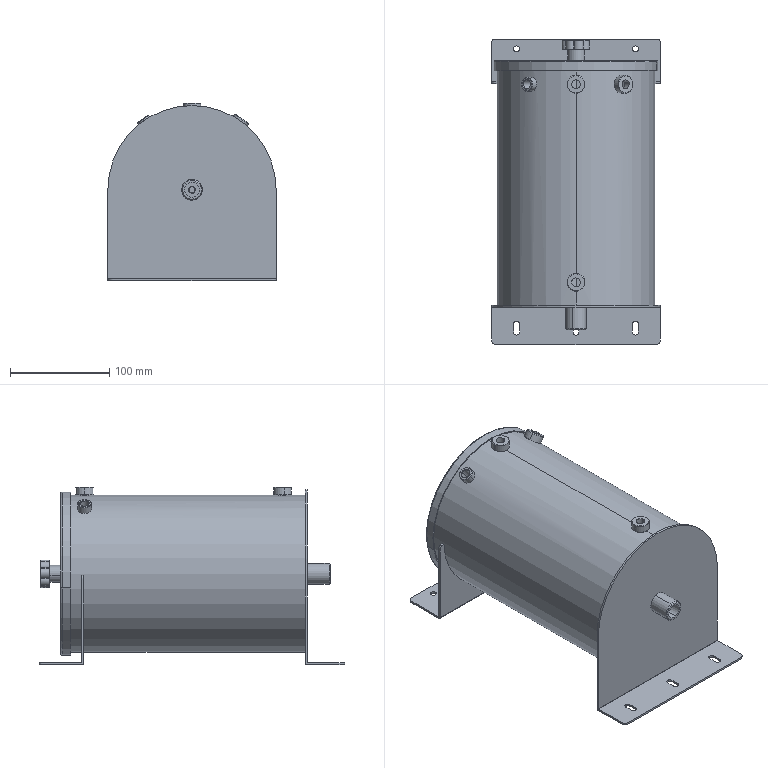Part | SolidWorks | 11 solids | 226 faces | box 170 x 309 x 179.5 mm | volume 403796 mm3 | cylinder 116 | plane 52 | spline 30 | cone 24 | torus 4 | commonest cylinder face diameters 6 x38 10 x12 1 x9 8.8 x8 12 x6 18 x6